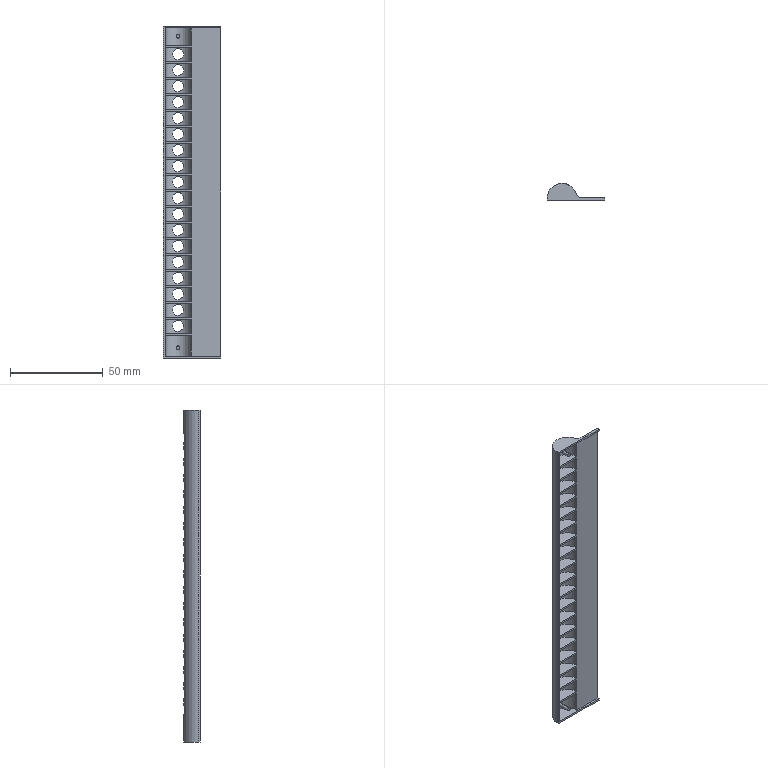Part | SolidWorks | features ICE 5, Fillet 2, Extrusion 1, Shell 1 | 1 solid | 114 faces | box 30.992 x 9 x 178.57 mm | volume 6725 mm3 | cylinder 63 | plane 51 | commonest cylinder face diameters 6 x37 14 x20 2 x4 1 x1 16 x1